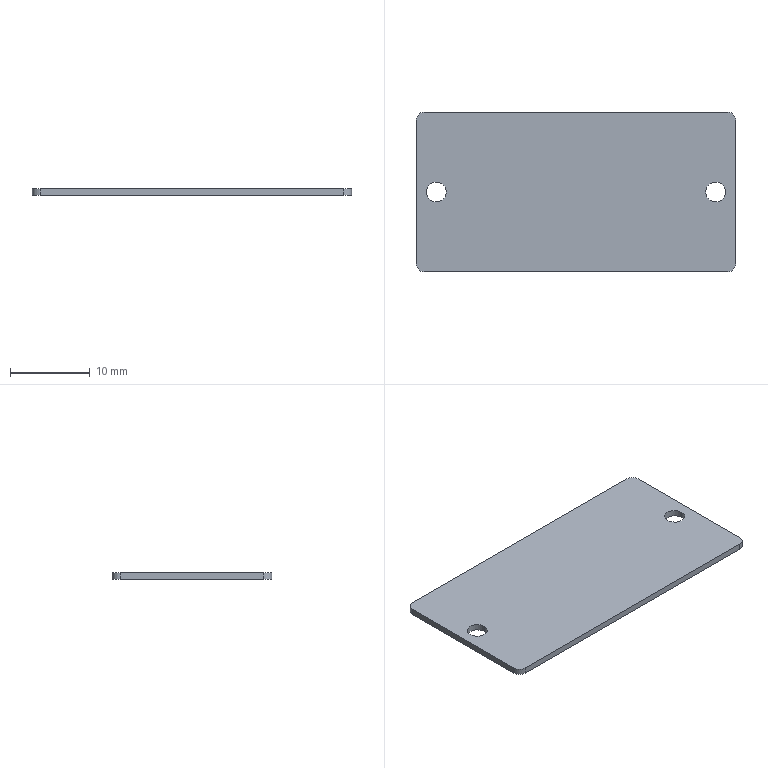Part | STEP file | J101-EBZ05-17-12-Part-3 | 1 solid | 14 faces | box 40 x 20 x 0.8 mm | volume 631.459 mm3 | cylinder 8 | plane 6 | commonest cylinder face diameters 2 x4 2.5 x4
STEP:
#1=CARTESIAN_POINT('',(0.,0.,0.));
#2=DIRECTION('',(0.,0.,1.));
#3=DIRECTION('',(1.,0.,0.));
#4=AXIS2_PLACEMENT_3D('',#1,#2,#3);
#5=CARTESIAN_POINT('',(-18.75,10.,0.));
#6=VERTEX_POINT('',#5);
#7=CARTESIAN_POINT('',(-18.75,10.,-0.8));
#8=VERTEX_POINT('',#7);
#9=CARTESIAN_POINT('',(-18.75,10.,0.));
#10=DIRECTION('',(0.,0.,-1.));
#11=VECTOR('',#10,1.);
#12=LINE('',#9,#11);
#13=CARTESIAN_POINT('',(-17.5,10.,0.));
#14=DIRECTION('',(0.,0.,-1.));
#15=DIRECTION('',(-1.,0.,0.));
#16=AXIS2_PLACEMENT_3D('',#13,#14,#15);
#17=CYLINDRICAL_SURFACE('',#16,1.25);
#18=CARTESIAN_POINT('',(6.283,0.));
#19=DIRECTION('',(0.,1.));
#20=VECTOR('',#19,1.);
#21=LINE('',#18,#20);
#22=(GEOMETRIC_REPRESENTATION_CONTEXT(2)PARAMETRIC_REPRESENTATION_CONTEXT()REPRESENTATION_CONTEXT('',''));
#23=DEFINITIONAL_REPRESENTATION('',(#21),#22);
#24=PCURVE('',#17,#23);
#25=CARTESIAN_POINT('',(-17.5,10.,0.));
#26=DIRECTION('',(0.,0.,-1.));
#27=DIRECTION('',(-1.,0.,0.));
#28=AXIS2_PLACEMENT_3D('',#25,#26,#27);
#29=CYLINDRICAL_SURFACE('',#28,1.25);
#30=CARTESIAN_POINT('',(0.,0.));
#31=DIRECTION('',(0.,1.));
#32=VECTOR('',#31,1.);
#33=LINE('',#30,#32);
#34=(GEOMETRIC_REPRESENTATION_CONTEXT(2)PARAMETRIC_REPRESENTATION_CONTEXT()REPRESENTATION_CONTEXT('',''));
#35=DEFINITIONAL_REPRESENTATION('',(#33),#34);
#36=PCURVE('',#29,#35);
#37=SURFACE_CURVE('',#12,(#24,#36),.PCURVE_S1.);
#38=EDGE_CURVE('',#6,#8,#37,.T.);
#39=ORIENTED_EDGE('',*,*,#38,.T.);
#40=CARTESIAN_POINT('',(-16.25,10.,-0.8));
#41=VERTEX_POINT('',#40);
#42=CARTESIAN_POINT('',(-17.5,10.,-0.8));
#43=DIRECTION('',(0.,0.,1.));
#44=DIRECTION('',(1.,0.,0.));
#45=AXIS2_PLACEMENT_3D('',#42,#43,#44);
#46=CIRCLE('',#45,1.25);
#47=CARTESIAN_POINT('',(9.425,0.8));
#48=DIRECTION('',(-1.,0.));
#49=VECTOR('',#48,1.);
#50=LINE('',#47,#49);
#51=(GEOMETRIC_REPRESENTATION_CONTEXT(2)PARAMETRIC_REPRESENTATION_CONTEXT()REPRESENTATION_CONTEXT('',''));
#52=DEFINITIONAL_REPRESENTATION('',(#50),#51);
#53=PCURVE('',#17,#52);
#54=CARTESIAN_POINT('',(19.,19.,-0.8));
#55=DIRECTION('',(0.,0.,1.));
#56=DIRECTION('',(1.,0.,0.));
#57=AXIS2_PLACEMENT_3D('',#54,#55,#56);
#58=PLANE('',#57);
#59=CARTESIAN_POINT('',(-36.5,-9.));
#60=DIRECTION('',(1.,0.));
#61=AXIS2_PLACEMENT_2D('',#59,#60);
#62=CIRCLE('',#61,1.25);
#63=(GEOMETRIC_REPRESENTATION_CONTEXT(2)PARAMETRIC_REPRESENTATION_CONTEXT()REPRESENTATION_CONTEXT('',''));
#64=DEFINITIONAL_REPRESENTATION('',(#62),#63);
#65=PCURVE('',#58,#64);
#66=SURFACE_CURVE('',#46,(#53,#65),.PCURVE_S1.);
#67=EDGE_CURVE('',#8,#41,#66,.T.);
#68=ORIENTED_EDGE('',*,*,#67,.T.);
#69=CARTESIAN_POINT('',(-16.25,10.,0.));
#70=VERTEX_POINT('',#69);
#71=CARTESIAN_POINT('',(-16.25,10.,0.));
#72=DIRECTION('',(0.,0.,-1.));
#73=VECTOR('',#72,1.);
#74=LINE('',#71,#73);
#75=CARTESIAN_POINT('',(3.142,0.));
#76=DIRECTION('',(0.,1.));
#77=VECTOR('',#76,1.);
#78=LINE('',#75,#77);
#79=(GEOMETRIC_REPRESENTATION_CONTEXT(2)PARAMETRIC_REPRESENTATION_CONTEXT()REPRESENTATION_CONTEXT('',''));
#80=DEFINITIONAL_REPRESENTATION('',(#78),#79);
#81=PCURVE('',#17,#80);
#82=CARTESIAN_POINT('',(3.142,0.));
#83=DIRECTION('',(0.,1.));
#84=VECTOR('',#83,1.);
#85=LINE('',#82,#84);
#86=(GEOMETRIC_REPRESENTATION_CONTEXT(2)PARAMETRIC_REPRESENTATION_CONTEXT()REPRESENTATION_CONTEXT('',''));
#87=DEFINITIONAL_REPRESENTATION('',(#85),#86);
#88=PCURVE('',#29,#87);
#89=SURFACE_CURVE('',#74,(#81,#88),.PCURVE_S1.);
#90=EDGE_CURVE('',#70,#41,#89,.T.);
#91=ORIENTED_EDGE('',*,*,#90,.F.);
#92=CARTESIAN_POINT('',(-17.5,10.,0.));
#93=DIRECTION('',(0.,0.,-1.));
#94=DIRECTION('',(-1.,0.,0.));
#95=AXIS2_PLACEMENT_3D('',#92,#93,#94);
#96=CIRCLE('',#95,1.25);
#97=CARTESIAN_POINT('',(0.,0.));
#98=DIRECTION('',(1.,0.));
#99=VECTOR('',#98,1.);
#100=LINE('',#97,#99);
#101=(GEOMETRIC_REPRESENTATION_CONTEXT(2)PARAMETRIC_REPRESENTATION_CONTEXT()REPRESENTATION_CONTEXT('',''));
#102=DEFINITIONAL_REPRESENTATION('',(#100),#101);
#103=PCURVE('',#17,#102);
#104=CARTESIAN_POINT('',(19.,19.,0.));
#105=DIRECTION('',(0.,0.,1.));
#106=DIRECTION('',(1.,0.,0.));
#107=AXIS2_PLACEMENT_3D('',#104,#105,#106);
#108=PLANE('',#107);
#109=CARTESIAN_POINT('',(-37.75,-9.));
#110=CARTESIAN_POINT('',(-37.75,-6.835));
#111=CARTESIAN_POINT('',(-35.875,-7.917));
#112=CARTESIAN_POINT('',(-34.,-9.));
#113=CARTESIAN_POINT('',(-35.875,-10.083));
#114=CARTESIAN_POINT('',(-37.75,-11.165));
#115=CARTESIAN_POINT('',(-37.75,-9.));
#116=(BOUNDED_CURVE()B_SPLINE_CURVE(2,(#109,#110,#111,#112,#113,#114,#115),.UNSPECIFIED.,.T.,.F.)B_SPLINE_CURVE_WITH_KNOTS((1,2,2,2,2,1),(-2.094,0.,2.094,4.189,6.283,8.378),.UNSPECIFIED.)CURVE()GEOMETRIC_REPRESENTATION_ITEM()RATIONAL_B_SPLINE_CURVE((1.,0.5,1.,0.5,1.,0.5,1.))REPRESENTATION_ITEM(''));
#117=(GEOMETRIC_REPRESENTATION_CONTEXT(2)PARAMETRIC_REPRESENTATION_CONTEXT()REPRESENTATION_CONTEXT('',''));
#118=DEFINITIONAL_REPRESENTATION('',(#116),#117);
#119=PCURVE('',#108,#118);
#120=SURFACE_CURVE('',#96,(#103,#119),.PCURVE_S1.);
#121=EDGE_CURVE('',#70,#6,#120,.T.);
#122=ORIENTED_EDGE('',*,*,#121,.T.);
#123=EDGE_LOOP('',(#39,#68,#91,#122));
#124=FACE_BOUND('',#123,.F.);
#125=ADVANCED_FACE('',(#124),#17,.F.);
#126=CARTESIAN_POINT('',(16.25,10.,0.));
#127=VERTEX_POINT('',#126);
#128=CARTESIAN_POINT('',(16.25,10.,-0.8));
#129=VERTEX_POINT('',#128);
#130=CARTESIAN_POINT('',(16.25,10.,0.));
#131=DIRECTION('',(0.,0.,-1.));
#132=VECTOR('',#131,1.);
#133=LINE('',#130,#132);
#134=CARTESIAN_POINT('',(17.5,10.,0.));
#135=DIRECTION('',(0.,0.,-1.));
#136=DIRECTION('',(-1.,0.,0.));
#137=AXIS2_PLACEMENT_3D('',#134,#135,#136);
#138=CYLINDRICAL_SURFACE('',#137,1.25);
#139=CARTESIAN_POINT('',(6.283,0.));
#140=DIRECTION('',(0.,1.));
#141=VECTOR('',#140,1.);
#142=LINE('',#139,#141);
#143=(GEOMETRIC_REPRESENTATION_CONTEXT(2)PARAMETRIC_REPRESENTATION_CONTEXT()REPRESENTATION_CONTEXT('',''));
#144=DEFINITIONAL_REPRESENTATION('',(#142),#143);
#145=PCURVE('',#138,#144);
#146=CARTESIAN_POINT('',(17.5,10.,0.));
#147=DIRECTION('',(0.,0.,-1.));
#148=DIRECTION('',(-1.,0.,0.));
#149=AXIS2_PLACEMENT_3D('',#146,#147,#148);
#150=CYLINDRICAL_SURFACE('',#149,1.25);
#151=CARTESIAN_POINT('',(0.,0.));
#152=DIRECTION('',(0.,1.));
#153=VECTOR('',#152,1.);
#154=LINE('',#151,#153);
#155=(GEOMETRIC_REPRESENTATION_CONTEXT(2)PARAMETRIC_REPRESENTATION_CONTEXT()REPRESENTATION_CONTEXT('',''));
#156=DEFINITIONAL_REPRESENTATION('',(#154),#155);
#157=PCURVE('',#150,#156);
#158=SURFACE_CURVE('',#133,(#145,#157),.PCURVE_S1.);
#159=EDGE_CURVE('',#127,#129,#158,.T.);
#160=ORIENTED_EDGE('',*,*,#159,.T.);
#161=CARTESIAN_POINT('',(18.75,10.,-0.8));
#162=VERTEX_POINT('',#161);
#163=CARTESIAN_POINT('',(17.5,10.,-0.8));
#164=DIRECTION('',(0.,0.,1.));
#165=DIRECTION('',(1.,0.,0.));
#166=AXIS2_PLACEMENT_3D('',#163,#164,#165);
#167=CIRCLE('',#166,1.25);
#168=CARTESIAN_POINT('',(9.425,0.8));
#169=DIRECTION('',(-1.,0.));
#170=VECTOR('',#169,1.);
#171=LINE('',#168,#170);
#172=(GEOMETRIC_REPRESENTATION_CONTEXT(2)PARAMETRIC_REPRESENTATION_CONTEXT()REPRESENTATION_CONTEXT('',''));
#173=DEFINITIONAL_REPRESENTATION('',(#171),#172);
#174=PCURVE('',#138,#173);
#175=CARTESIAN_POINT('',(-1.5,-9.));
#176=DIRECTION('',(1.,0.));
#177=AXIS2_PLACEMENT_2D('',#175,#176);
#178=CIRCLE('',#177,1.25);
#179=(GEOMETRIC_REPRESENTATION_CONTEXT(2)PARAMETRIC_REPRESENTATION_CONTEXT()REPRESENTATION_CONTEXT('',''));
#180=DEFINITIONAL_REPRESENTATION('',(#178),#179);
#181=PCURVE('',#58,#180);
#182=SURFACE_CURVE('',#167,(#174,#181),.PCURVE_S1.);
#183=EDGE_CURVE('',#129,#162,#182,.T.);
#184=ORIENTED_EDGE('',*,*,#183,.T.);
#185=CARTESIAN_POINT('',(18.75,10.,0.));
#186=VERTEX_POINT('',#185);
#187=CARTESIAN_POINT('',(18.75,10.,0.));
#188=DIRECTION('',(0.,0.,-1.));
#189=VECTOR('',#188,1.);
#190=LINE('',#187,#189);
#191=CARTESIAN_POINT('',(3.142,0.));
#192=DIRECTION('',(0.,1.));
#193=VECTOR('',#192,1.);
#194=LINE('',#191,#193);
#195=(GEOMETRIC_REPRESENTATION_CONTEXT(2)PARAMETRIC_REPRESENTATION_CONTEXT()REPRESENTATION_CONTEXT('',''));
#196=DEFINITIONAL_REPRESENTATION('',(#194),#195);
#197=PCURVE('',#138,#196);
#198=CARTESIAN_POINT('',(3.142,0.));
#199=DIRECTION('',(0.,1.));
#200=VECTOR('',#199,1.);
#201=LINE('',#198,#200);
#202=(GEOMETRIC_REPRESENTATION_CONTEXT(2)PARAMETRIC_REPRESENTATION_CONTEXT()REPRESENTATION_CONTEXT('',''));
#203=DEFINITIONAL_REPRESENTATION('',(#201),#202);
#204=PCURVE('',#150,#203);
#205=SURFACE_CURVE('',#190,(#197,#204),.PCURVE_S1.);
#206=EDGE_CURVE('',#186,#162,#205,.T.);
#207=ORIENTED_EDGE('',*,*,#206,.F.);
#208=CARTESIAN_POINT('',(17.5,10.,0.));
#209=DIRECTION('',(0.,0.,-1.));
#210=DIRECTION('',(-1.,0.,0.));
#211=AXIS2_PLACEMENT_3D('',#208,#209,#210);
#212=CIRCLE('',#211,1.25);
#213=CARTESIAN_POINT('',(0.,0.));
#214=DIRECTION('',(1.,0.));
#215=VECTOR('',#214,1.);
#216=LINE('',#213,#215);
#217=(GEOMETRIC_REPRESENTATION_CONTEXT(2)PARAMETRIC_REPRESENTATION_CONTEXT()REPRESENTATION_CONTEXT('',''));
#218=DEFINITIONAL_REPRESENTATION('',(#216),#217);
#219=PCURVE('',#138,#218);
#220=CARTESIAN_POINT('',(-2.75,-9.));
#221=CARTESIAN_POINT('',(-2.75,-6.835));
#222=CARTESIAN_POINT('',(-0.875,-7.917));
#223=CARTESIAN_POINT('',(1.,-9.));
#224=CARTESIAN_POINT('',(-0.875,-10.083));
#225=CARTESIAN_POINT('',(-2.75,-11.165));
#226=CARTESIAN_POINT('',(-2.75,-9.));
#227=(BOUNDED_CURVE()B_SPLINE_CURVE(2,(#220,#221,#222,#223,#224,#225,#226),.UNSPECIFIED.,.T.,.F.)B_SPLINE_CURVE_WITH_KNOTS((1,2,2,2,2,1),(-2.094,0.,2.094,4.189,6.283,8.378),.UNSPECIFIED.)CURVE()GEOMETRIC_REPRESENTATION_ITEM()RATIONAL_B_SPLINE_CURVE((1.,0.5,1.,0.5,1.,0.5,1.))REPRESENTATION_ITEM(''));
#228=(GEOMETRIC_REPRESENTATION_CONTEXT(2)PARAMETRIC_REPRESENTATION_CONTEXT()REPRESENTATION_CONTEXT('',''));
#229=DEFINITIONAL_REPRESENTATION('',(#227),#228);
#230=PCURVE('',#108,#229);
#231=SURFACE_CURVE('',#212,(#219,#230),.PCURVE_S1.);
#232=EDGE_CURVE('',#186,#127,#231,.T.);
#233=ORIENTED_EDGE('',*,*,#232,.T.);
#234=EDGE_LOOP('',(#160,#184,#207,#233));
#235=FACE_BOUND('',#234,.F.);
#236=ADVANCED_FACE('',(#235),#138,.F.);
#237=CARTESIAN_POINT('',(20.,19.,0.));
#238=VERTEX_POINT('',#237);
#239=CARTESIAN_POINT('',(19.,20.,0.));
#240=VERTEX_POINT('',#239);
#241=CARTESIAN_POINT('',(19.,19.,0.));
#242=DIRECTION('',(0.,0.,1.));
#243=DIRECTION('',(1.,0.,0.));
#244=AXIS2_PLACEMENT_3D('',#241,#242,#243);
#245=CIRCLE('',#244,1.);
#246=CARTESIAN_POINT('',(19.,19.,-0.8));
#247=DIRECTION('',(0.,0.,1.));
#248=DIRECTION('',(1.,0.,0.));
#249=AXIS2_PLACEMENT_3D('',#246,#247,#248);
#250=CYLINDRICAL_SURFACE('',#249,1.);
#251=CARTESIAN_POINT('',(0.,0.8));
#252=DIRECTION('',(1.,0.));
#253=VECTOR('',#252,1.);
#254=LINE('',#251,#253);
#255=(GEOMETRIC_REPRESENTATION_CONTEXT(2)PARAMETRIC_REPRESENTATION_CONTEXT()REPRESENTATION_CONTEXT('',''));
#256=DEFINITIONAL_REPRESENTATION('',(#254),#255);
#257=PCURVE('',#250,#256);
#258=CARTESIAN_POINT('',(0.,0.));
#259=DIRECTION('',(1.,0.));
#260=AXIS2_PLACEMENT_2D('',#258,#259);
#261=CIRCLE('',#260,1.);
#262=(GEOMETRIC_REPRESENTATION_CONTEXT(2)PARAMETRIC_REPRESENTATION_CONTEXT()REPRESENTATION_CONTEXT('',''));
#263=DEFINITIONAL_REPRESENTATION('',(#261),#262);
#264=PCURVE('',#108,#263);
#265=SURFACE_CURVE('',#245,(#257,#264),.PCURVE_S1.);
#266=EDGE_CURVE('',#238,#240,#265,.T.);
#267=ORIENTED_EDGE('',*,*,#266,.F.);
#268=CARTESIAN_POINT('',(20.,19.,-0.8));
#269=VERTEX_POINT('',#268);
#270=CARTESIAN_POINT('',(20.,19.,-0.8));
#271=DIRECTION('',(0.,0.,1.));
#272=VECTOR('',#271,1.);
#273=LINE('',#270,#272);
#274=CARTESIAN_POINT('',(0.,0.));
#275=DIRECTION('',(0.,1.));
#276=VECTOR('',#275,1.);
#277=LINE('',#274,#276);
#278=(GEOMETRIC_REPRESENTATION_CONTEXT(2)PARAMETRIC_REPRESENTATION_CONTEXT()REPRESENTATION_CONTEXT('',''));
#279=DEFINITIONAL_REPRESENTATION('',(#277),#278);
#280=PCURVE('',#250,#279);
#281=CARTESIAN_POINT('',(20.,1.,-0.8));
#282=DIRECTION('',(1.,0.,0.));
#283=DIRECTION('',(0.,0.,-1.));
#284=AXIS2_PLACEMENT_3D('',#281,#282,#283);
#285=PLANE('',#284);
#286=CARTESIAN_POINT('',(0.,18.));
#287=DIRECTION('',(-1.,0.));
#288=VECTOR('',#287,1.);
#289=LINE('',#286,#288);
#290=(GEOMETRIC_REPRESENTATION_CONTEXT(2)PARAMETRIC_REPRESENTATION_CONTEXT()REPRESENTATION_CONTEXT('',''));
#291=DEFINITIONAL_REPRESENTATION('',(#289),#290);
#292=PCURVE('',#285,#291);
#293=SURFACE_CURVE('',#273,(#280,#292),.PCURVE_S1.);
#294=EDGE_CURVE('',#269,#238,#293,.T.);
#295=ORIENTED_EDGE('',*,*,#294,.F.);
#296=CARTESIAN_POINT('',(19.,20.,-0.8));
#297=VERTEX_POINT('',#296);
#298=CARTESIAN_POINT('',(19.,19.,-0.8));
#299=DIRECTION('',(0.,0.,1.));
#300=DIRECTION('',(1.,0.,0.));
#301=AXIS2_PLACEMENT_3D('',#298,#299,#300);
#302=CIRCLE('',#301,1.);
#303=CARTESIAN_POINT('',(0.,0.));
#304=DIRECTION('',(1.,0.));
#305=VECTOR('',#304,1.);
#306=LINE('',#303,#305);
#307=(GEOMETRIC_REPRESENTATION_CONTEXT(2)PARAMETRIC_REPRESENTATION_CONTEXT()REPRESENTATION_CONTEXT('',''));
#308=DEFINITIONAL_REPRESENTATION('',(#306),#307);
#309=PCURVE('',#250,#308);
#310=CARTESIAN_POINT('',(0.,0.));
#311=DIRECTION('',(1.,0.));
#312=AXIS2_PLACEMENT_2D('',#310,#311);
#313=CIRCLE('',#312,1.);
#314=(GEOMETRIC_REPRESENTATION_CONTEXT(2)PARAMETRIC_REPRESENTATION_CONTEXT()REPRESENTATION_CONTEXT('',''));
#315=DEFINITIONAL_REPRESENTATION('',(#313),#314);
#316=PCURVE('',#58,#315);
#317=SURFACE_CURVE('',#302,(#309,#316),.PCURVE_S1.);
#318=EDGE_CURVE('',#269,#297,#317,.T.);
#319=ORIENTED_EDGE('',*,*,#318,.T.);
#320=CARTESIAN_POINT('',(19.,20.,-0.8));
#321=DIRECTION('',(0.,0.,1.));
#322=VECTOR('',#321,1.);
#323=LINE('',#320,#322);
#324=CARTESIAN_POINT('',(1.571,0.));
#325=DIRECTION('',(0.,1.));
#326=VECTOR('',#325,1.);
#327=LINE('',#324,#326);
#328=(GEOMETRIC_REPRESENTATION_CONTEXT(2)PARAMETRIC_REPRESENTATION_CONTEXT()REPRESENTATION_CONTEXT('',''));
#329=DEFINITIONAL_REPRESENTATION('',(#327),#328);
#330=PCURVE('',#250,#329);
#331=CARTESIAN_POINT('',(19.,20.,-0.8));
#332=DIRECTION('',(0.,1.,0.));
#333=DIRECTION('',(-1.,0.,0.));
#334=AXIS2_PLACEMENT_3D('',#331,#332,#333);
#335=PLANE('',#334);
#336=CARTESIAN_POINT('',(0.,0.));
#337=DIRECTION('',(0.,1.));
#338=VECTOR('',#337,1.);
#339=LINE('',#336,#338);
#340=(GEOMETRIC_REPRESENTATION_CONTEXT(2)PARAMETRIC_REPRESENTATION_CONTEXT()REPRESENTATION_CONTEXT('',''));
#341=DEFINITIONAL_REPRESENTATION('',(#339),#340);
#342=PCURVE('',#335,#341);
#343=SURFACE_CURVE('',#323,(#330,#342),.PCURVE_S1.);
#344=EDGE_CURVE('',#297,#240,#343,.T.);
#345=ORIENTED_EDGE('',*,*,#344,.T.);
#346=EDGE_LOOP('',(#267,#295,#319,#345));
#347=FACE_BOUND('',#346,.T.);
#348=ADVANCED_FACE('',(#347),#250,.T.);
#349=CARTESIAN_POINT('',(-19.,20.,0.));
#350=VERTEX_POINT('',#349);
#351=CARTESIAN_POINT('',(19.,20.,0.));
#352=DIRECTION('',(-1.,0.,0.));
#353=VECTOR('',#352,1.);
#354=LINE('',#351,#353);
#355=CARTESIAN_POINT('',(0.,0.8));
#356=DIRECTION('',(1.,0.));
#357=VECTOR('',#356,1.);
#358=LINE('',#355,#357);
#359=(GEOMETRIC_REPRESENTATION_CONTEXT(2)PARAMETRIC_REPRESENTATION_CONTEXT()REPRESENTATION_CONTEXT('',''));
#360=DEFINITIONAL_REPRESENTATION('',(#358),#359);
#361=PCURVE('',#335,#360);
#362=CARTESIAN_POINT('',(0.,1.));
#363=DIRECTION('',(-1.,0.));
#364=VECTOR('',#363,1.);
#365=LINE('',#362,#364);
#366=(GEOMETRIC_REPRESENTATION_CONTEXT(2)PARAMETRIC_REPRESENTATION_CONTEXT()REPRESENTATION_CONTEXT('',''));
#367=DEFINITIONAL_REPRESENTATION('',(#365),#366);
#368=PCURVE('',#108,#367);
#369=SURFACE_CURVE('',#354,(#361,#368),.PCURVE_S1.);
#370=EDGE_CURVE('',#240,#350,#369,.T.);
#371=ORIENTED_EDGE('',*,*,#370,.F.);
#372=ORIENTED_EDGE('',*,*,#344,.F.);
#373=CARTESIAN_POINT('',(-19.,20.,-0.8));
#374=VERTEX_POINT('',#373);
#375=CARTESIAN_POINT('',(19.,20.,-0.8));
#376=DIRECTION('',(-1.,0.,0.));
#377=VECTOR('',#376,1.);
#378=LINE('',#375,#377);
#379=CARTESIAN_POINT('',(0.,0.));
#380=DIRECTION('',(1.,0.));
#381=VECTOR('',#380,1.);
#382=LINE('',#379,#381);
#383=(GEOMETRIC_REPRESENTATION_CONTEXT(2)PARAMETRIC_REPRESENTATION_CONTEXT()REPRESENTATION_CONTEXT('',''));
#384=DEFINITIONAL_REPRESENTATION('',(#382),#383);
#385=PCURVE('',#335,#384);
#386=CARTESIAN_POINT('',(0.,1.));
#387=DIRECTION('',(-1.,0.));
#388=VECTOR('',#387,1.);
#389=LINE('',#386,#388);
#390=(GEOMETRIC_REPRESENTATION_CONTEXT(2)PARAMETRIC_REPRESENTATION_CONTEXT()REPRESENTATION_CONTEXT('',''));
#391=DEFINITIONAL_REPRESENTATION('',(#389),#390);
#392=PCURVE('',#58,#391);
#393=SURFACE_CURVE('',#378,(#385,#392),.PCURVE_S1.);
#394=EDGE_CURVE('',#297,#374,#393,.T.);
#395=ORIENTED_EDGE('',*,*,#394,.T.);
#396=CARTESIAN_POINT('',(-19.,20.,-0.8));
#397=DIRECTION('',(0.,0.,1.));
#398=VECTOR('',#397,1.);
#399=LINE('',#396,#398);
#400=CARTESIAN_POINT('',(38.,0.));
#401=DIRECTION('',(0.,1.));
#402=VECTOR('',#401,1.);
#403=LINE('',#400,#402);
#404=(GEOMETRIC_REPRESENTATION_CONTEXT(2)PARAMETRIC_REPRESENTATION_CONTEXT()REPRESENTATION_CONTEXT('',''));
#405=DEFINITIONAL_REPRESENTATION('',(#403),#404);
#406=PCURVE('',#335,#405);
#407=CARTESIAN_POINT('',(-19.,19.,-0.8));
#408=DIRECTION('',(0.,0.,1.));
#409=DIRECTION('',(1.,0.,0.));
#410=AXIS2_PLACEMENT_3D('',#407,#408,#409);
#411=CYLINDRICAL_SURFACE('',#410,1.);
#412=CARTESIAN_POINT('',(1.571,0.));
#413=DIRECTION('',(0.,1.));
#414=VECTOR('',#413,1.);
#415=LINE('',#412,#414);
#416=(GEOMETRIC_REPRESENTATION_CONTEXT(2)PARAMETRIC_REPRESENTATION_CONTEXT()REPRESENTATION_CONTEXT('',''));
#417=DEFINITIONAL_REPRESENTATION('',(#415),#416);
#418=PCURVE('',#411,#417);
#419=SURFACE_CURVE('',#399,(#406,#418),.PCURVE_S1.);
#420=EDGE_CURVE('',#374,#350,#419,.T.);
#421=ORIENTED_EDGE('',*,*,#420,.T.);
#422=EDGE_LOOP('',(#371,#372,#395,#421));
#423=FACE_BOUND('',#422,.T.);
#424=ADVANCED_FACE('',(#423),#335,.T.);
#425=CARTESIAN_POINT('',(-20.,19.,0.));
#426=VERTEX_POINT('',#425);
#427=CARTESIAN_POINT('',(-19.,19.,0.));
#428=DIRECTION('',(0.,0.,1.));
#429=DIRECTION('',(1.,0.,0.));
#430=AXIS2_PLACEMENT_3D('',#427,#428,#429);
#431=CIRCLE('',#430,1.);
#432=CARTESIAN_POINT('',(0.,0.8));
#433=DIRECTION('',(1.,0.));
#434=VECTOR('',#433,1.);
#435=LINE('',#432,#434);
#436=(GEOMETRIC_REPRESENTATION_CONTEXT(2)PARAMETRIC_REPRESENTATION_CONTEXT()REPRESENTATION_CONTEXT('',''));
#437=DEFINITIONAL_REPRESENTATION('',(#435),#436);
#438=PCURVE('',#411,#437);
#439=CARTESIAN_POINT('',(-38.,0.));
#440=DIRECTION('',(1.,0.));
#441=AXIS2_PLACEMENT_2D('',#439,#440);
#442=CIRCLE('',#441,1.);
#443=(GEOMETRIC_REPRESENTATION_CONTEXT(2)PARAMETRIC_REPRESENTATION_CONTEXT()REPRESENTATION_CONTEXT('',''));
#444=DEFINITIONAL_REPRESENTATION('',(#442),#443);
#445=PCURVE('',#108,#444);
#446=SURFACE_CURVE('',#431,(#438,#445),.PCURVE_S1.);
#447=EDGE_CURVE('',#350,#426,#446,.T.);
#448=ORIENTED_EDGE('',*,*,#447,.F.);
#449=ORIENTED_EDGE('',*,*,#420,.F.);
#450=CARTESIAN_POINT('',(-20.,19.,-0.8));
#451=VERTEX_POINT('',#450);
#452=CARTESIAN_POINT('',(-19.,19.,-0.8));
#453=DIRECTION('',(0.,0.,1.));
#454=DIRECTION('',(1.,0.,0.));
#455=AXIS2_PLACEMENT_3D('',#452,#453,#454);
#456=CIRCLE('',#455,1.);
#457=CARTESIAN_POINT('',(0.,0.));
#458=DIRECTION('',(1.,0.));
#459=VECTOR('',#458,1.);
#460=LINE('',#457,#459);
#461=(GEOMETRIC_REPRESENTATION_CONTEXT(2)PARAMETRIC_REPRESENTATION_CONTEXT()REPRESENTATION_CONTEXT('',''));
#462=DEFINITIONAL_REPRESENTATION('',(#460),#461);
#463=PCURVE('',#411,#462);
#464=CARTESIAN_POINT('',(-38.,0.));
#465=DIRECTION('',(1.,0.));
#466=AXIS2_PLACEMENT_2D('',#464,#465);
#467=CIRCLE('',#466,1.);
#468=(GEOMETRIC_REPRESENTATION_CONTEXT(2)PARAMETRIC_REPRESENTATION_CONTEXT()REPRESENTATION_CONTEXT('',''));
#469=DEFINITIONAL_REPRESENTATION('',(#467),#468);
#470=PCURVE('',#58,#469);
#471=SURFACE_CURVE('',#456,(#463,#470),.PCURVE_S1.);
#472=EDGE_CURVE('',#374,#451,#471,.T.);
#473=ORIENTED_EDGE('',*,*,#472,.T.);
#474=CARTESIAN_POINT('',(-20.,19.,-0.8));
#475=DIRECTION('',(0.,0.,1.));
#476=VECTOR('',#475,1.);
#477=LINE('',#474,#476);
#478=CARTESIAN_POINT('',(3.142,0.));
#479=DIRECTION('',(0.,1.));
#480=VECTOR('',#479,1.);
#481=LINE('',#478,#480);
#482=(GEOMETRIC_REPRESENTATION_CONTEXT(2)PARAMETRIC_REPRESENTATION_CONTEXT()REPRESENTATION_CONTEXT('',''));
#483=DEFINITIONAL_REPRESENTATION('',(#481),#482);
#484=PCURVE('',#411,#483);
#485=CARTESIAN_POINT('',(-20.,19.,-0.8));
#486=DIRECTION('',(-1.,0.,0.));
#487=DIRECTION('',(0.,-1.,0.));
#488=AXIS2_PLACEMENT_3D('',#485,#486,#487);
#489=PLANE('',#488);
#490=CARTESIAN_POINT('',(0.,0.));
#491=DIRECTION('',(0.,1.));
#492=VECTOR('',#491,1.);
#493=LINE('',#490,#492);
#494=(GEOMETRIC_REPRESENTATION_CONTEXT(2)PARAMETRIC_REPRESENTATION_CONTEXT()REPRESENTATION_CONTEXT('',''));
#495=DEFINITIONAL_REPRESENTATION('',(#493),#494);
#496=PCURVE('',#489,#495);
#497=SURFACE_CURVE('',#477,(#484,#496),.PCURVE_S1.);
#498=EDGE_CURVE('',#451,#426,#497,.T.);
#499=ORIENTED_EDGE('',*,*,#498,.T.);
#500=EDGE_LOOP('',(#448,#449,#473,#499));
#501=FACE_BOUND('',#500,.T.);
#502=ADVANCED_FACE('',(#501),#411,.T.);
#503=CARTESIAN_POINT('',(-20.,1.,0.));
#504=VERTEX_POINT('',#503);
#505=CARTESIAN_POINT('',(-20.,19.,0.));
#506=DIRECTION('',(0.,-1.,0.));
#507=VECTOR('',#506,1.);
#508=LINE('',#505,#507);
#509=CARTESIAN_POINT('',(0.,0.8));
#510=DIRECTION('',(1.,0.));
#511=VECTOR('',#510,1.);
#512=LINE('',#509,#511);
#513=(GEOMETRIC_REPRESENTATION_CONTEXT(2)PARAMETRIC_REPRESENTATION_CONTEXT()REPRESENTATION_CONTEXT('',''));
#514=DEFINITIONAL_REPRESENTATION('',(#512),#513);
#515=PCURVE('',#489,#514);
#516=CARTESIAN_POINT('',(-39.,0.));
#517=DIRECTION('',(0.,-1.));
#518=VECTOR('',#517,1.);
#519=LINE('',#516,#518);
#520=(GEOMETRIC_REPRESENTATION_CONTEXT(2)PARAMETRIC_REPRESENTATION_CONTEXT()REPRESENTATION_CONTEXT('',''));
#521=DEFINITIONAL_REPRESENTATION('',(#519),#520);
#522=PCURVE('',#108,#521);
#523=SURFACE_CURVE('',#508,(#515,#522),.PCURVE_S1.);
#524=EDGE_CURVE('',#426,#504,#523,.T.);
#525=ORIENTED_EDGE('',*,*,#524,.F.);
#526=ORIENTED_EDGE('',*,*,#498,.F.);
#527=CARTESIAN_POINT('',(-20.,1.,-0.8));
#528=VERTEX_POINT('',#527);
#529=CARTESIAN_POINT('',(-20.,19.,-0.8));
#530=DIRECTION('',(0.,-1.,0.));
#531=VECTOR('',#530,1.);
#532=LINE('',#529,#531);
#533=CARTESIAN_POINT('',(0.,0.));
#534=DIRECTION('',(1.,0.));
#535=VECTOR('',#534,1.);
#536=LINE('',#533,#535);
#537=(GEOMETRIC_REPRESENTATION_CONTEXT(2)PARAMETRIC_REPRESENTATION_CONTEXT()REPRESENTATION_CONTEXT('',''));
#538=DEFINITIONAL_REPRESENTATION('',(#536),#537);
#539=PCURVE('',#489,#538);
#540=CARTESIAN_POINT('',(-39.,0.));
#541=DIRECTION('',(0.,-1.));
#542=VECTOR('',#541,1.);
#543=LINE('',#540,#542);
#544=(GEOMETRIC_REPRESENTATION_CONTEXT(2)PARAMETRIC_REPRESENTATION_CONTEXT()REPRESENTATION_CONTEXT('',''));
#545=DEFINITIONAL_REPRESENTATION('',(#543),#544);
#546=PCURVE('',#58,#545);
#547=SURFACE_CURVE('',#532,(#539,#546),.PCURVE_S1.);
#548=EDGE_CURVE('',#451,#528,#547,.T.);
#549=ORIENTED_EDGE('',*,*,#548,.T.);
#550=CARTESIAN_POINT('',(-20.,1.,-0.8));
#551=DIRECTION('',(0.,0.,1.));
#552=VECTOR('',#551,1.);
#553=LINE('',#550,#552);
#554=CARTESIAN_POINT('',(18.,0.));
#555=DIRECTION('',(0.,1.));
#556=VECTOR('',#555,1.);
#557=LINE('',#554,#556);
#558=(GEOMETRIC_REPRESENTATION_CONTEXT(2)PARAMETRIC_REPRESENTATION_CONTEXT()REPRESENTATION_CONTEXT('',''));
#559=DEFINITIONAL_REPRESENTATION('',(#557),#558);
#560=PCURVE('',#489,#559);
#561=CARTESIAN_POINT('',(-19.,1.,-0.8));
#562=DIRECTION('',(0.,0.,1.));
#563=DIRECTION('',(1.,0.,0.));
#564=AXIS2_PLACEMENT_3D('',#561,#562,#563);
#565=CYLINDRICAL_SURFACE('',#564,1.);
#566=CARTESIAN_POINT('',(3.142,0.));
#567=DIRECTION('',(0.,1.));
#568=VECTOR('',#567,1.);
#569=LINE('',#566,#568);
#570=(GEOMETRIC_REPRESENTATION_CONTEXT(2)PARAMETRIC_REPRESENTATION_CONTEXT()REPRESENTATION_CONTEXT('',''));
#571=DEFINITIONAL_REPRESENTATION('',(#569),#570);
#572=PCURVE('',#565,#571);
#573=SURFACE_CURVE('',#553,(#560,#572),.PCURVE_S1.);
#574=EDGE_CURVE('',#528,#504,#573,.T.);
#575=ORIENTED_EDGE('',*,*,#574,.T.);
#576=EDGE_LOOP('',(#525,#526,#549,#575));
#577=FACE_BOUND('',#576,.T.);
#578=ADVANCED_FACE('',(#577),#489,.T.);
#579=CARTESIAN_POINT('',(-19.,0.,0.));
#580=VERTEX_POINT('',#579);
#581=CARTESIAN_POINT('',(-19.,1.,0.));
#582=DIRECTION('',(0.,0.,1.));
#583=DIRECTION('',(1.,0.,0.));
#584=AXIS2_PLACEMENT_3D('',#581,#582,#583);
#585=CIRCLE('',#584,1.);
#586=CARTESIAN_POINT('',(0.,0.8));
#587=DIRECTION('',(1.,0.));
#588=VECTOR('',#587,1.);
#589=LINE('',#586,#588);
#590=(GEOMETRIC_REPRESENTATION_CONTEXT(2)PARAMETRIC_REPRESENTATION_CONTEXT()REPRESENTATION_CONTEXT('',''));
#591=DEFINITIONAL_REPRESENTATION('',(#589),#590);
#592=PCURVE('',#565,#591);
#593=CARTESIAN_POINT('',(-38.,-18.));
#594=DIRECTION('',(1.,0.));
#595=AXIS2_PLACEMENT_2D('',#593,#594);
#596=CIRCLE('',#595,1.);
#597=(GEOMETRIC_REPRESENTATION_CONTEXT(2)PARAMETRIC_REPRESENTATION_CONTEXT()REPRESENTATION_CONTEXT('',''));
#598=DEFINITIONAL_REPRESENTATION('',(#596),#597);
#599=PCURVE('',#108,#598);
#600=SURFACE_CURVE('',#585,(#592,#599),.PCURVE_S1.);
#601=EDGE_CURVE('',#504,#580,#600,.T.);
#602=ORIENTED_EDGE('',*,*,#601,.F.);
#603=ORIENTED_EDGE('',*,*,#574,.F.);
#604=CARTESIAN_POINT('',(-19.,0.,-0.8));
#605=VERTEX_POINT('',#604);
#606=CARTESIAN_POINT('',(-19.,1.,-0.8));
#607=DIRECTION('',(0.,0.,1.));
#608=DIRECTION('',(1.,0.,0.));
#609=AXIS2_PLACEMENT_3D('',#606,#607,#608);
#610=CIRCLE('',#609,1.);
#611=CARTESIAN_POINT('',(0.,0.));
#612=DIRECTION('',(1.,0.));
#613=VECTOR('',#612,1.);
#614=LINE('',#611,#613);
#615=(GEOMETRIC_REPRESENTATION_CONTEXT(2)PARAMETRIC_REPRESENTATION_CONTEXT()REPRESENTATION_CONTEXT('',''));
#616=DEFINITIONAL_REPRESENTATION('',(#614),#615);
#617=PCURVE('',#565,#616);
#618=CARTESIAN_POINT('',(-38.,-18.));
#619=DIRECTION('',(1.,0.));
#620=AXIS2_PLACEMENT_2D('',#618,#619);
#621=CIRCLE('',#620,1.);
#622=(GEOMETRIC_REPRESENTATION_CONTEXT(2)PARAMETRIC_REPRESENTATION_CONTEXT()REPRESENTATION_CONTEXT('',''));
#623=DEFINITIONAL_REPRESENTATION('',(#621),#622);
#624=PCURVE('',#58,#623);
#625=SURFACE_CURVE('',#610,(#617,#624),.PCURVE_S1.);
#626=EDGE_CURVE('',#528,#605,#625,.T.);
#627=ORIENTED_EDGE('',*,*,#626,.T.);
#628=CARTESIAN_POINT('',(-19.,0.,-0.8));
#629=DIRECTION('',(0.,0.,1.));
#630=VECTOR('',#629,1.);
#631=LINE('',#628,#630);
#632=CARTESIAN_POINT('',(4.712,0.));
#633=DIRECTION('',(0.,1.));
#634=VECTOR('',#633,1.);
#635=LINE('',#632,#634);
#636=(GEOMETRIC_REPRESENTATION_CONTEXT(2)PARAMETRIC_REPRESENTATION_CONTEXT()REPRESENTATION_CONTEXT('',''));
#637=DEFINITIONAL_REPRESENTATION('',(#635),#636);
#638=PCURVE('',#565,#637);
#639=CARTESIAN_POINT('',(-19.,0.,-0.8));
#640=DIRECTION('',(0.,-1.,0.));
#641=DIRECTION('',(1.,0.,0.));
#642=AXIS2_PLACEMENT_3D('',#639,#640,#641);
#643=PLANE('',#642);
#644=CARTESIAN_POINT('',(0.,0.));
#645=DIRECTION('',(0.,1.));
#646=VECTOR('',#645,1.);
#647=LINE('',#644,#646);
#648=(GEOMETRIC_REPRESENTATION_CONTEXT(2)PARAMETRIC_REPRESENTATION_CONTEXT()REPRESENTATION_CONTEXT('',''));
#649=DEFINITIONAL_REPRESENTATION('',(#647),#648);
#650=PCURVE('',#643,#649);
#651=SURFACE_CURVE('',#631,(#638,#650),.PCURVE_S1.);
#652=EDGE_CURVE('',#605,#580,#651,.T.);
#653=ORIENTED_EDGE('',*,*,#652,.T.);
#654=EDGE_LOOP('',(#602,#603,#627,#653));
#655=FACE_BOUND('',#654,.T.);
#656=ADVANCED_FACE('',(#655),#565,.T.);
#657=CARTESIAN_POINT('',(19.,0.,0.));
#658=VERTEX_POINT('',#657);
#659=CARTESIAN_POINT('',(-19.,0.,0.));
#660=DIRECTION('',(1.,0.,0.));
#661=VECTOR('',#660,1.);
#662=LINE('',#659,#661);
#663=CARTESIAN_POINT('',(0.,0.8));
#664=DIRECTION('',(1.,0.));
#665=VECTOR('',#664,1.);
#666=LINE('',#663,#665);
#667=(GEOMETRIC_REPRESENTATION_CONTEXT(2)PARAMETRIC_REPRESENTATION_CONTEXT()REPRESENTATION_CONTEXT('',''));
#668=DEFINITIONAL_REPRESENTATION('',(#666),#667);
#669=PCURVE('',#643,#668);
#670=CARTESIAN_POINT('',(-38.,-19.));
#671=DIRECTION('',(1.,0.));
#672=VECTOR('',#671,1.);
#673=LINE('',#670,#672);
#674=(GEOMETRIC_REPRESENTATION_CONTEXT(2)PARAMETRIC_REPRESENTATION_CONTEXT()REPRESENTATION_CONTEXT('',''));
#675=DEFINITIONAL_REPRESENTATION('',(#673),#674);
#676=PCURVE('',#108,#675);
#677=SURFACE_CURVE('',#662,(#669,#676),.PCURVE_S1.);
#678=EDGE_CURVE('',#580,#658,#677,.T.);
#679=ORIENTED_EDGE('',*,*,#678,.F.);
#680=ORIENTED_EDGE('',*,*,#652,.F.);
#681=CARTESIAN_POINT('',(19.,0.,-0.8));
#682=VERTEX_POINT('',#681);
#683=CARTESIAN_POINT('',(-19.,0.,-0.8));
#684=DIRECTION('',(1.,0.,0.));
#685=VECTOR('',#684,1.);
#686=LINE('',#683,#685);
#687=CARTESIAN_POINT('',(0.,0.));
#688=DIRECTION('',(1.,0.));
#689=VECTOR('',#688,1.);
#690=LINE('',#687,#689);
#691=(GEOMETRIC_REPRESENTATION_CONTEXT(2)PARAMETRIC_REPRESENTATION_CONTEXT()REPRESENTATION_CONTEXT('',''));
#692=DEFINITIONAL_REPRESENTATION('',(#690),#691);
#693=PCURVE('',#643,#692);
#694=CARTESIAN_POINT('',(-38.,-19.));
#695=DIRECTION('',(1.,0.));
#696=VECTOR('',#695,1.);
#697=LINE('',#694,#696);
#698=(GEOMETRIC_REPRESENTATION_CONTEXT(2)PARAMETRIC_REPRESENTATION_CONTEXT()REPRESENTATION_CONTEXT('',''));
#699=DEFINITIONAL_REPRESENTATION('',(#697),#698);
#700=PCURVE('',#58,#699);
#701=SURFACE_CURVE('',#686,(#693,#700),.PCURVE_S1.);
#702=EDGE_CURVE('',#605,#682,#701,.T.);
#703=ORIENTED_EDGE('',*,*,#702,.T.);
#704=CARTESIAN_POINT('',(19.,0.,-0.8));
#705=DIRECTION('',(0.,0.,1.));
#706=VECTOR('',#705,1.);
#707=LINE('',#704,#706);
#708=CARTESIAN_POINT('',(38.,0.));
#709=DIRECTION('',(0.,1.));
#710=VECTOR('',#709,1.);
#711=LINE('',#708,#710);
#712=(GEOMETRIC_REPRESENTATION_CONTEXT(2)PARAMETRIC_REPRESENTATION_CONTEXT()REPRESENTATION_CONTEXT('',''));
#713=DEFINITIONAL_REPRESENTATION('',(#711),#712);
#714=PCURVE('',#643,#713);
#715=CARTESIAN_POINT('',(19.,1.,-0.8));
#716=DIRECTION('',(0.,0.,1.));
#717=DIRECTION('',(1.,0.,0.));
#718=AXIS2_PLACEMENT_3D('',#715,#716,#717);
#719=CYLINDRICAL_SURFACE('',#718,1.);
#720=CARTESIAN_POINT('',(4.712,0.));
#721=DIRECTION('',(0.,1.));
#722=VECTOR('',#721,1.);
#723=LINE('',#720,#722);
#724=(GEOMETRIC_REPRESENTATION_CONTEXT(2)PARAMETRIC_REPRESENTATION_CONTEXT()REPRESENTATION_CONTEXT('',''));
#725=DEFINITIONAL_REPRESENTATION('',(#723),#724);
#726=PCURVE('',#719,#725);
#727=SURFACE_CURVE('',#707,(#714,#726),.PCURVE_S1.);
#728=EDGE_CURVE('',#682,#658,#727,.T.);
#729=ORIENTED_EDGE('',*,*,#728,.T.);
#730=EDGE_LOOP('',(#679,#680,#703,#729));
#731=FACE_BOUND('',#730,.T.);
#732=ADVANCED_FACE('',(#731),#643,.T.);
#733=CARTESIAN_POINT('',(20.,1.,0.));
#734=VERTEX_POINT('',#733);
#735=CARTESIAN_POINT('',(19.,1.,0.));
#736=DIRECTION('',(0.,0.,1.));
#737=DIRECTION('',(1.,0.,0.));
#738=AXIS2_PLACEMENT_3D('',#735,#736,#737);
#739=CIRCLE('',#738,1.);
#740=CARTESIAN_POINT('',(0.,0.8));
#741=DIRECTION('',(1.,0.));
#742=VECTOR('',#741,1.);
#743=LINE('',#740,#742);
#744=(GEOMETRIC_REPRESENTATION_CONTEXT(2)PARAMETRIC_REPRESENTATION_CONTEXT()REPRESENTATION_CONTEXT('',''));
#745=DEFINITIONAL_REPRESENTATION('',(#743),#744);
#746=PCURVE('',#719,#745);
#747=CARTESIAN_POINT('',(0.,-18.));
#748=DIRECTION('',(1.,0.));
#749=AXIS2_PLACEMENT_2D('',#747,#748);
#750=CIRCLE('',#749,1.);
#751=(GEOMETRIC_REPRESENTATION_CONTEXT(2)PARAMETRIC_REPRESENTATION_CONTEXT()REPRESENTATION_CONTEXT('',''));
#752=DEFINITIONAL_REPRESENTATION('',(#750),#751);
#753=PCURVE('',#108,#752);
#754=SURFACE_CURVE('',#739,(#746,#753),.PCURVE_S1.);
#755=EDGE_CURVE('',#658,#734,#754,.T.);
#756=ORIENTED_EDGE('',*,*,#755,.F.);
#757=ORIENTED_EDGE('',*,*,#728,.F.);
#758=CARTESIAN_POINT('',(20.,1.,-0.8));
#759=VERTEX_POINT('',#758);
#760=CARTESIAN_POINT('',(19.,1.,-0.8));
#761=DIRECTION('',(0.,0.,1.));
#762=DIRECTION('',(1.,0.,0.));
#763=AXIS2_PLACEMENT_3D('',#760,#761,#762);
#764=CIRCLE('',#763,1.);
#765=CARTESIAN_POINT('',(0.,0.));
#766=DIRECTION('',(1.,0.));
#767=VECTOR('',#766,1.);
#768=LINE('',#765,#767);
#769=(GEOMETRIC_REPRESENTATION_CONTEXT(2)PARAMETRIC_REPRESENTATION_CONTEXT()REPRESENTATION_CONTEXT('',''));
#770=DEFINITIONAL_REPRESENTATION('',(#768),#769);
#771=PCURVE('',#719,#770);
#772=CARTESIAN_POINT('',(0.,-18.));
#773=DIRECTION('',(1.,0.));
#774=AXIS2_PLACEMENT_2D('',#772,#773);
#775=CIRCLE('',#774,1.);
#776=(GEOMETRIC_REPRESENTATION_CONTEXT(2)PARAMETRIC_REPRESENTATION_CONTEXT()REPRESENTATION_CONTEXT('',''));
#777=DEFINITIONAL_REPRESENTATION('',(#775),#776);
#778=PCURVE('',#58,#777);
#779=SURFACE_CURVE('',#764,(#771,#778),.PCURVE_S1.);
#780=EDGE_CURVE('',#682,#759,#779,.T.);
#781=ORIENTED_EDGE('',*,*,#780,.T.);
#782=CARTESIAN_POINT('',(20.,1.,-0.8));
#783=DIRECTION('',(0.,0.,1.));
#784=VECTOR('',#783,1.);
#785=LINE('',#782,#784);
#786=CARTESIAN_POINT('',(6.283,0.));
#787=DIRECTION('',(0.,1.));
#788=VECTOR('',#787,1.);
#789=LINE('',#786,#788);
#790=(GEOMETRIC_REPRESENTATION_CONTEXT(2)PARAMETRIC_REPRESENTATION_CONTEXT()REPRESENTATION_CONTEXT('',''));
#791=DEFINITIONAL_REPRESENTATION('',(#789),#790);
#792=PCURVE('',#719,#791);
#793=CARTESIAN_POINT('',(0.,0.));
#794=DIRECTION('',(-1.,0.));
#795=VECTOR('',#794,1.);
#796=LINE('',#793,#795);
#797=(GEOMETRIC_REPRESENTATION_CONTEXT(2)PARAMETRIC_REPRESENTATION_CONTEXT()REPRESENTATION_CONTEXT('',''));
#798=DEFINITIONAL_REPRESENTATION('',(#796),#797);
#799=PCURVE('',#285,#798);
#800=SURFACE_CURVE('',#785,(#792,#799),.PCURVE_S1.);
#801=EDGE_CURVE('',#759,#734,#800,.T.);
#802=ORIENTED_EDGE('',*,*,#801,.T.);
#803=EDGE_LOOP('',(#756,#757,#781,#802));
#804=FACE_BOUND('',#803,.T.);
#805=ADVANCED_FACE('',(#804),#719,.T.);
#806=CARTESIAN_POINT('',(20.,1.,0.));
#807=DIRECTION('',(0.,1.,0.));
#808=VECTOR('',#807,1.);
#809=LINE('',#806,#808);
#810=CARTESIAN_POINT('',(-0.8,0.));
#811=DIRECTION('',(0.,1.));
#812=VECTOR('',#811,1.);
#813=LINE('',#810,#812);
#814=(GEOMETRIC_REPRESENTATION_CONTEXT(2)PARAMETRIC_REPRESENTATION_CONTEXT()REPRESENTATION_CONTEXT('',''));
#815=DEFINITIONAL_REPRESENTATION('',(#813),#814);
#816=PCURVE('',#285,#815);
#817=CARTESIAN_POINT('',(1.,-18.));
#818=DIRECTION('',(0.,1.));
#819=VECTOR('',#818,1.);
#820=LINE('',#817,#819);
#821=(GEOMETRIC_REPRESENTATION_CONTEXT(2)PARAMETRIC_REPRESENTATION_CONTEXT()REPRESENTATION_CONTEXT('',''));
#822=DEFINITIONAL_REPRESENTATION('',(#820),#821);
#823=PCURVE('',#108,#822);
#824=SURFACE_CURVE('',#809,(#816,#823),.PCURVE_S1.);
#825=EDGE_CURVE('',#734,#238,#824,.T.);
#826=ORIENTED_EDGE('',*,*,#825,.F.);
#827=ORIENTED_EDGE('',*,*,#801,.F.);
#828=CARTESIAN_POINT('',(20.,1.,-0.8));
#829=DIRECTION('',(0.,1.,0.));
#830=VECTOR('',#829,1.);
#831=LINE('',#828,#830);
#832=CARTESIAN_POINT('',(0.,0.));
#833=DIRECTION('',(0.,1.));
#834=VECTOR('',#833,1.);
#835=LINE('',#832,#834);
#836=(GEOMETRIC_REPRESENTATION_CONTEXT(2)PARAMETRIC_REPRESENTATION_CONTEXT()REPRESENTATION_CONTEXT('',''));
#837=DEFINITIONAL_REPRESENTATION('',(#835),#836);
#838=PCURVE('',#285,#837);
#839=CARTESIAN_POINT('',(1.,-18.));
#840=DIRECTION('',(0.,1.));
#841=VECTOR('',#840,1.);
#842=LINE('',#839,#841);
#843=(GEOMETRIC_REPRESENTATION_CONTEXT(2)PARAMETRIC_REPRESENTATION_CONTEXT()REPRESENTATION_CONTEXT('',''));
#844=DEFINITIONAL_REPRESENTATION('',(#842),#843);
#845=PCURVE('',#58,#844);
#846=SURFACE_CURVE('',#831,(#838,#845),.PCURVE_S1.);
#847=EDGE_CURVE('',#759,#269,#846,.T.);
#848=ORIENTED_EDGE('',*,*,#847,.T.);
#849=ORIENTED_EDGE('',*,*,#294,.T.);
#850=EDGE_LOOP('',(#826,#827,#848,#849));
#851=FACE_BOUND('',#850,.T.);
#852=ADVANCED_FACE('',(#851),#285,.T.);
#853=ORIENTED_EDGE('',*,*,#67,.T.);
#854=CARTESIAN_POINT('',(-17.5,10.,-0.8));
#855=DIRECTION('',(0.,0.,1.));
#856=DIRECTION('',(1.,0.,0.));
#857=AXIS2_PLACEMENT_3D('',#854,#855,#856);
#858=CIRCLE('',#857,1.25);
#859=CARTESIAN_POINT('',(-36.5,-9.));
#860=DIRECTION('',(1.,0.));
#861=AXIS2_PLACEMENT_2D('',#859,#860);
#862=CIRCLE('',#861,1.25);
#863=(GEOMETRIC_REPRESENTATION_CONTEXT(2)PARAMETRIC_REPRESENTATION_CONTEXT()REPRESENTATION_CONTEXT('',''));
#864=DEFINITIONAL_REPRESENTATION('',(#862),#863);
#865=PCURVE('',#58,#864);
#866=CARTESIAN_POINT('',(3.142,0.8));
#867=DIRECTION('',(-1.,0.));
#868=VECTOR('',#867,1.);
#869=LINE('',#866,#868);
#870=(GEOMETRIC_REPRESENTATION_CONTEXT(2)PARAMETRIC_REPRESENTATION_CONTEXT()REPRESENTATION_CONTEXT('',''));
#871=DEFINITIONAL_REPRESENTATION('',(#869),#870);
#872=PCURVE('',#29,#871);
#873=SURFACE_CURVE('',#858,(#865,#872),.PCURVE_S1.);
#874=EDGE_CURVE('',#41,#8,#873,.T.);
#875=ORIENTED_EDGE('',*,*,#874,.T.);
#876=EDGE_LOOP('',(#853,#875));
#877=FACE_BOUND('',#876,.T.);
#878=ORIENTED_EDGE('',*,*,#183,.T.);
#879=CARTESIAN_POINT('',(17.5,10.,-0.8));
#880=DIRECTION('',(0.,0.,1.));
#881=DIRECTION('',(1.,0.,0.));
#882=AXIS2_PLACEMENT_3D('',#879,#880,#881);
#883=CIRCLE('',#882,1.25);
#884=CARTESIAN_POINT('',(-1.5,-9.));
#885=DIRECTION('',(1.,0.));
#886=AXIS2_PLACEMENT_2D('',#884,#885);
#887=CIRCLE('',#886,1.25);
#888=(GEOMETRIC_REPRESENTATION_CONTEXT(2)PARAMETRIC_REPRESENTATION_CONTEXT()REPRESENTATION_CONTEXT('',''));
#889=DEFINITIONAL_REPRESENTATION('',(#887),#888);
#890=PCURVE('',#58,#889);
#891=CARTESIAN_POINT('',(3.142,0.8));
#892=DIRECTION('',(-1.,0.));
#893=VECTOR('',#892,1.);
#894=LINE('',#891,#893);
#895=(GEOMETRIC_REPRESENTATION_CONTEXT(2)PARAMETRIC_REPRESENTATION_CONTEXT()REPRESENTATION_CONTEXT('',''));
#896=DEFINITIONAL_REPRESENTATION('',(#894),#895);
#897=PCURVE('',#150,#896);
#898=SURFACE_CURVE('',#883,(#890,#897),.PCURVE_S1.);
#899=EDGE_CURVE('',#162,#129,#898,.T.);
#900=ORIENTED_EDGE('',*,*,#899,.T.);
#901=EDGE_LOOP('',(#878,#900));
#902=FACE_BOUND('',#901,.T.);
#903=ORIENTED_EDGE('',*,*,#318,.F.);
#904=ORIENTED_EDGE('',*,*,#847,.F.);
#905=ORIENTED_EDGE('',*,*,#780,.F.);
#906=ORIENTED_EDGE('',*,*,#702,.F.);
#907=ORIENTED_EDGE('',*,*,#626,.F.);
#908=ORIENTED_EDGE('',*,*,#548,.F.);
#909=ORIENTED_EDGE('',*,*,#472,.F.);
#910=ORIENTED_EDGE('',*,*,#394,.F.);
#911=EDGE_LOOP('',(#903,#904,#905,#906,#907,#908,#909,#910));
#912=FACE_BOUND('',#911,.T.);
#913=ADVANCED_FACE('',(#877,#902,#912),#58,.F.);
#914=CARTESIAN_POINT('',(-17.5,10.,0.));
#915=DIRECTION('',(0.,0.,-1.));
#916=DIRECTION('',(-1.,0.,0.));
#917=AXIS2_PLACEMENT_3D('',#914,#915,#916);
#918=CIRCLE('',#917,1.25);
#919=CARTESIAN_POINT('',(-37.75,-9.));
#920=CARTESIAN_POINT('',(-37.75,-6.835));
#921=CARTESIAN_POINT('',(-35.875,-7.917));
#922=CARTESIAN_POINT('',(-34.,-9.));
#923=CARTESIAN_POINT('',(-35.875,-10.083));
#924=CARTESIAN_POINT('',(-37.75,-11.165));
#925=CARTESIAN_POINT('',(-37.75,-9.));
#926=(BOUNDED_CURVE()B_SPLINE_CURVE(2,(#919,#920,#921,#922,#923,#924,#925),.UNSPECIFIED.,.T.,.F.)B_SPLINE_CURVE_WITH_KNOTS((1,2,2,2,2,1),(-2.094,0.,2.094,4.189,6.283,8.378),.UNSPECIFIED.)CURVE()GEOMETRIC_REPRESENTATION_ITEM()RATIONAL_B_SPLINE_CURVE((1.,0.5,1.,0.5,1.,0.5,1.))REPRESENTATION_ITEM(''));
#927=(GEOMETRIC_REPRESENTATION_CONTEXT(2)PARAMETRIC_REPRESENTATION_CONTEXT()REPRESENTATION_CONTEXT('',''));
#928=DEFINITIONAL_REPRESENTATION('',(#926),#927);
#929=PCURVE('',#108,#928);
#930=CARTESIAN_POINT('',(0.,0.));
#931=DIRECTION('',(1.,0.));
#932=VECTOR('',#931,1.);
#933=LINE('',#930,#932);
#934=(GEOMETRIC_REPRESENTATION_CONTEXT(2)PARAMETRIC_REPRESENTATION_CONTEXT()REPRESENTATION_CONTEXT('',''));
#935=DEFINITIONAL_REPRESENTATION('',(#933),#934);
#936=PCURVE('',#29,#935);
#937=SURFACE_CURVE('',#918,(#929,#936),.PCURVE_S1.);
#938=EDGE_CURVE('',#6,#70,#937,.T.);
#939=ORIENTED_EDGE('',*,*,#938,.T.);
#940=ORIENTED_EDGE('',*,*,#121,.T.);
#941=EDGE_LOOP('',(#939,#940));
#942=FACE_BOUND('',#941,.T.);
#943=CARTESIAN_POINT('',(17.5,10.,0.));
#944=DIRECTION('',(0.,0.,-1.));
#945=DIRECTION('',(-1.,0.,0.));
#946=AXIS2_PLACEMENT_3D('',#943,#944,#945);
#947=CIRCLE('',#946,1.25);
#948=CARTESIAN_POINT('',(-2.75,-9.));
#949=CARTESIAN_POINT('',(-2.75,-6.835));
#950=CARTESIAN_POINT('',(-0.875,-7.917));
#951=CARTESIAN_POINT('',(1.,-9.));
#952=CARTESIAN_POINT('',(-0.875,-10.083));
#953=CARTESIAN_POINT('',(-2.75,-11.165));
#954=CARTESIAN_POINT('',(-2.75,-9.));
#955=(BOUNDED_CURVE()B_SPLINE_CURVE(2,(#948,#949,#950,#951,#952,#953,#954),.UNSPECIFIED.,.T.,.F.)B_SPLINE_CURVE_WITH_KNOTS((1,2,2,2,2,1),(-2.094,0.,2.094,4.189,6.283,8.378),.UNSPECIFIED.)CURVE()GEOMETRIC_REPRESENTATION_ITEM()RATIONAL_B_SPLINE_CURVE((1.,0.5,1.,0.5,1.,0.5,1.))REPRESENTATION_ITEM(''));
#956=(GEOMETRIC_REPRESENTATION_CONTEXT(2)PARAMETRIC_REPRESENTATION_CONTEXT()REPRESENTATION_CONTEXT('',''));
#957=DEFINITIONAL_REPRESENTATION('',(#955),#956);
#958=PCURVE('',#108,#957);
#959=CARTESIAN_POINT('',(0.,0.));
#960=DIRECTION('',(1.,0.));
#961=VECTOR('',#960,1.);
#962=LINE('',#959,#961);
#963=(GEOMETRIC_REPRESENTATION_CONTEXT(2)PARAMETRIC_REPRESENTATION_CONTEXT()REPRESENTATION_CONTEXT('',''));
#964=DEFINITIONAL_REPRESENTATION('',(#962),#963);
#965=PCURVE('',#150,#964);
#966=SURFACE_CURVE('',#947,(#958,#965),.PCURVE_S1.);
#967=EDGE_CURVE('',#127,#186,#966,.T.);
#968=ORIENTED_EDGE('',*,*,#967,.T.);
#969=ORIENTED_EDGE('',*,*,#232,.T.);
#970=EDGE_LOOP('',(#968,#969));
#971=FACE_BOUND('',#970,.T.);
#972=ORIENTED_EDGE('',*,*,#266,.T.);
#973=ORIENTED_EDGE('',*,*,#370,.T.);
#974=ORIENTED_EDGE('',*,*,#447,.T.);
#975=ORIENTED_EDGE('',*,*,#524,.T.);
#976=ORIENTED_EDGE('',*,*,#601,.T.);
#977=ORIENTED_EDGE('',*,*,#678,.T.);
#978=ORIENTED_EDGE('',*,*,#755,.T.);
#979=ORIENTED_EDGE('',*,*,#825,.T.);
#980=EDGE_LOOP('',(#972,#973,#974,#975,#976,#977,#978,#979));
#981=FACE_BOUND('',#980,.T.);
#982=ADVANCED_FACE('',(#942,#971,#981),#108,.T.);
#983=ORIENTED_EDGE('',*,*,#899,.T.);
#984=ORIENTED_EDGE('',*,*,#159,.F.);
#985=ORIENTED_EDGE('',*,*,#967,.T.);
#986=ORIENTED_EDGE('',*,*,#206,.T.);
#987=EDGE_LOOP('',(#983,#984,#985,#986));
#988=FACE_BOUND('',#987,.F.);
#989=ADVANCED_FACE('',(#988),#150,.F.);
#990=ORIENTED_EDGE('',*,*,#874,.T.);
#991=ORIENTED_EDGE('',*,*,#38,.F.);
#992=ORIENTED_EDGE('',*,*,#938,.T.);
#993=ORIENTED_EDGE('',*,*,#90,.T.);
#994=EDGE_LOOP('',(#990,#991,#992,#993));
#995=FACE_BOUND('',#994,.F.);
#996=ADVANCED_FACE('',(#995),#29,.F.);
#997=CLOSED_SHELL('',(#125,#236,#348,#424,#502,#578,#656,#732,#805,#852,#913,#982,#989,#996));
#998=MANIFOLD_SOLID_BREP('',#997);
#999=(LENGTH_UNIT()NAMED_UNIT(*)SI_UNIT(.MILLI.,.METRE.));
#1000=UNCERTAINTY_MEASURE_WITH_UNIT(LENGTH_MEASURE(0.0000001),#999,'','');
#1001=(NAMED_UNIT(*)PLANE_ANGLE_UNIT()SI_UNIT($,.RADIAN.));
#1002=(NAMED_UNIT(*)SI_UNIT($,.STERADIAN.)SOLID_ANGLE_UNIT());
#1003=(GEOMETRIC_REPRESENTATION_CONTEXT(3)GLOBAL_UNCERTAINTY_ASSIGNED_CONTEXT((#1000))GLOBAL_UNIT_ASSIGNED_CONTEXT((#999,#1001,#1002))REPRESENTATION_CONTEXT('',''));
#1004=ADVANCED_BREP_SHAPE_REPRESENTATION('',(#4,#998),#1003);